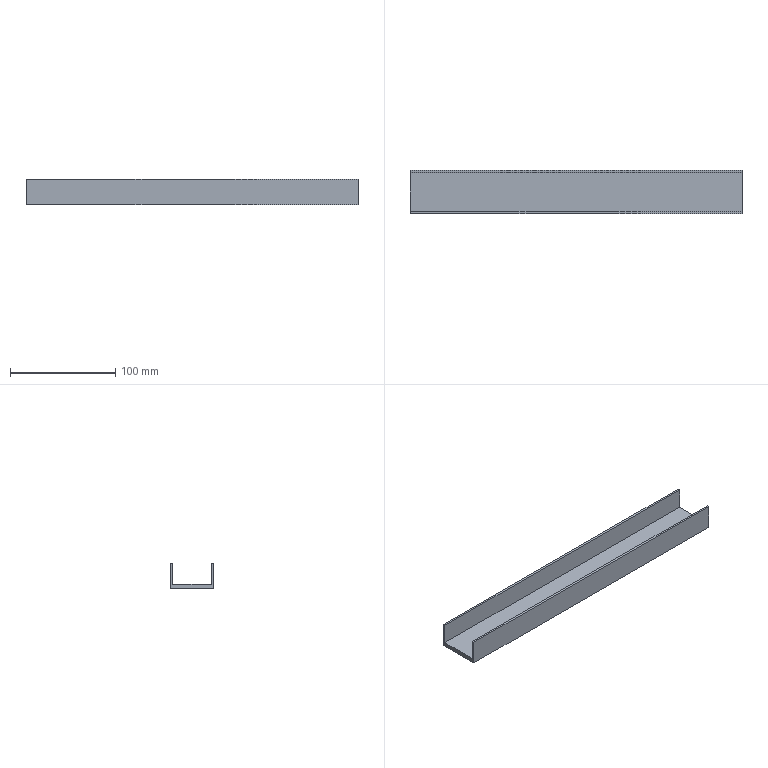Part | STEP file | Material chute | 1 solid | 10 faces | box 315 x 41 x 24 mm | volume 76860 mm3 | plane 10
STEP:
#1=CARTESIAN_POINT('',(190.,4.5,0.));
#2=VERTEX_POINT('',#1);
#3=CARTESIAN_POINT('',(190.,45.5,0.));
#4=VERTEX_POINT('',#3);
#5=CARTESIAN_POINT('',(190.,45.5,0.));
#6=DIRECTION('',(0.,1.,0.));
#7=VECTOR('',#6,1000.);
#8=LINE('',#5,#7);
#9=EDGE_CURVE('',#2,#4,#8,.T.);
#10=ORIENTED_EDGE('',*,*,#9,.T.);
#11=CARTESIAN_POINT('',(190.,45.5,24.));
#12=VERTEX_POINT('',#11);
#13=CARTESIAN_POINT('',(190.,45.5,4.));
#14=DIRECTION('',(0.,0.,-1.));
#15=VECTOR('',#14,1000.);
#16=LINE('',#13,#15);
#17=EDGE_CURVE('',#12,#4,#16,.T.);
#18=ORIENTED_EDGE('',*,*,#17,.F.);
#19=CARTESIAN_POINT('',(190.,43.5,24.));
#20=VERTEX_POINT('',#19);
#21=CARTESIAN_POINT('',(190.,45.5,24.));
#22=DIRECTION('',(0.,-1.,0.));
#23=VECTOR('',#22,1000.);
#24=LINE('',#21,#23);
#25=EDGE_CURVE('',#12,#20,#24,.T.);
#26=ORIENTED_EDGE('',*,*,#25,.T.);
#27=CARTESIAN_POINT('',(190.,43.5,4.));
#28=VERTEX_POINT('',#27);
#29=CARTESIAN_POINT('',(190.,43.5,24.));
#30=DIRECTION('',(0.,0.,-1.));
#31=VECTOR('',#30,1000.);
#32=LINE('',#29,#31);
#33=EDGE_CURVE('',#20,#28,#32,.T.);
#34=ORIENTED_EDGE('',*,*,#33,.T.);
#35=CARTESIAN_POINT('',(190.,6.5,4.));
#36=VERTEX_POINT('',#35);
#37=CARTESIAN_POINT('',(190.,45.5,4.));
#38=DIRECTION('',(0.,1.,0.));
#39=VECTOR('',#38,1000.);
#40=LINE('',#37,#39);
#41=EDGE_CURVE('',#36,#28,#40,.T.);
#42=ORIENTED_EDGE('',*,*,#41,.F.);
#43=CARTESIAN_POINT('',(190.,6.5,24.));
#44=VERTEX_POINT('',#43);
#45=CARTESIAN_POINT('',(190.,6.5,24.));
#46=DIRECTION('',(0.,0.,1.));
#47=VECTOR('',#46,1000.);
#48=LINE('',#45,#47);
#49=EDGE_CURVE('',#36,#44,#48,.T.);
#50=ORIENTED_EDGE('',*,*,#49,.T.);
#51=CARTESIAN_POINT('',(190.,4.5,24.));
#52=VERTEX_POINT('',#51);
#53=CARTESIAN_POINT('',(190.,4.5,24.));
#54=DIRECTION('',(0.,-1.,0.));
#55=VECTOR('',#54,1000.);
#56=LINE('',#53,#55);
#57=EDGE_CURVE('',#44,#52,#56,.T.);
#58=ORIENTED_EDGE('',*,*,#57,.T.);
#59=CARTESIAN_POINT('',(190.,4.5,4.));
#60=DIRECTION('',(0.,0.,-1.));
#61=VECTOR('',#60,1000.);
#62=LINE('',#59,#61);
#63=EDGE_CURVE('',#52,#2,#62,.T.);
#64=ORIENTED_EDGE('',*,*,#63,.T.);
#65=EDGE_LOOP('',(#10,#18,#26,#34,#42,#50,#58,#64));
#66=FACE_OUTER_BOUND('',#65,.T.);
#67=CARTESIAN_POINT('',(190.,45.5,4.));
#68=DIRECTION('',(-1.,0.,0.));
#69=DIRECTION('',(0.,0.,1.));
#70=AXIS2_PLACEMENT_3D('',#67,#68,#69);
#71=PLANE('',#70);
#72=ADVANCED_FACE('',(#66),#71,.F.);
#73=CARTESIAN_POINT('',(-125.,45.5,0.));
#74=VERTEX_POINT('',#73);
#75=CARTESIAN_POINT('',(190.,45.5,0.));
#76=DIRECTION('',(-1.,0.,0.));
#77=VECTOR('',#76,1000.);
#78=LINE('',#75,#77);
#79=EDGE_CURVE('',#4,#74,#78,.T.);
#80=ORIENTED_EDGE('',*,*,#79,.T.);
#81=CARTESIAN_POINT('',(-125.,45.5,24.));
#82=VERTEX_POINT('',#81);
#83=CARTESIAN_POINT('',(-125.,45.5,4.));
#84=DIRECTION('',(0.,0.,-1.));
#85=VECTOR('',#84,1000.);
#86=LINE('',#83,#85);
#87=EDGE_CURVE('',#82,#74,#86,.T.);
#88=ORIENTED_EDGE('',*,*,#87,.F.);
#89=CARTESIAN_POINT('',(210.1,45.5,24.));
#90=DIRECTION('',(-1.,0.,0.));
#91=VECTOR('',#90,1000.);
#92=LINE('',#89,#91);
#93=EDGE_CURVE('',#12,#82,#92,.T.);
#94=ORIENTED_EDGE('',*,*,#93,.F.);
#95=ORIENTED_EDGE('',*,*,#17,.T.);
#96=EDGE_LOOP('',(#80,#88,#94,#95));
#97=FACE_OUTER_BOUND('',#96,.T.);
#98=CARTESIAN_POINT('',(190.,45.5,4.));
#99=DIRECTION('',(0.,-1.,0.));
#100=DIRECTION('',(1.,0.,0.));
#101=AXIS2_PLACEMENT_3D('',#98,#99,#100);
#102=PLANE('',#101);
#103=ADVANCED_FACE('',(#97),#102,.F.);
#104=CARTESIAN_POINT('',(-125.,4.5,0.));
#105=VERTEX_POINT('',#104);
#106=CARTESIAN_POINT('',(-125.,45.5,0.));
#107=DIRECTION('',(0.,-1.,0.));
#108=VECTOR('',#107,1000.);
#109=LINE('',#106,#108);
#110=EDGE_CURVE('',#74,#105,#109,.T.);
#111=ORIENTED_EDGE('',*,*,#110,.T.);
#112=CARTESIAN_POINT('',(-125.,4.5,24.));
#113=VERTEX_POINT('',#112);
#114=CARTESIAN_POINT('',(-125.,4.5,4.));
#115=DIRECTION('',(0.,0.,-1.));
#116=VECTOR('',#115,1000.);
#117=LINE('',#114,#116);
#118=EDGE_CURVE('',#113,#105,#117,.T.);
#119=ORIENTED_EDGE('',*,*,#118,.F.);
#120=CARTESIAN_POINT('',(-125.,6.5,24.));
#121=VERTEX_POINT('',#120);
#122=CARTESIAN_POINT('',(-125.,4.5,24.));
#123=DIRECTION('',(0.,1.,0.));
#124=VECTOR('',#123,1000.);
#125=LINE('',#122,#124);
#126=EDGE_CURVE('',#113,#121,#125,.T.);
#127=ORIENTED_EDGE('',*,*,#126,.T.);
#128=CARTESIAN_POINT('',(-125.,6.5,4.));
#129=VERTEX_POINT('',#128);
#130=CARTESIAN_POINT('',(-125.,6.5,24.));
#131=DIRECTION('',(0.,0.,-1.));
#132=VECTOR('',#131,1000.);
#133=LINE('',#130,#132);
#134=EDGE_CURVE('',#121,#129,#133,.T.);
#135=ORIENTED_EDGE('',*,*,#134,.T.);
#136=CARTESIAN_POINT('',(-125.,43.5,4.));
#137=VERTEX_POINT('',#136);
#138=CARTESIAN_POINT('',(-125.,45.5,4.));
#139=DIRECTION('',(0.,-1.,0.));
#140=VECTOR('',#139,1000.);
#141=LINE('',#138,#140);
#142=EDGE_CURVE('',#137,#129,#141,.T.);
#143=ORIENTED_EDGE('',*,*,#142,.F.);
#144=CARTESIAN_POINT('',(-125.,43.5,24.));
#145=VERTEX_POINT('',#144);
#146=CARTESIAN_POINT('',(-125.,43.5,24.));
#147=DIRECTION('',(0.,0.,1.));
#148=VECTOR('',#147,1000.);
#149=LINE('',#146,#148);
#150=EDGE_CURVE('',#137,#145,#149,.T.);
#151=ORIENTED_EDGE('',*,*,#150,.T.);
#152=CARTESIAN_POINT('',(-125.,45.5,24.));
#153=DIRECTION('',(0.,1.,0.));
#154=VECTOR('',#153,1000.);
#155=LINE('',#152,#154);
#156=EDGE_CURVE('',#145,#82,#155,.T.);
#157=ORIENTED_EDGE('',*,*,#156,.T.);
#158=ORIENTED_EDGE('',*,*,#87,.T.);
#159=EDGE_LOOP('',(#111,#119,#127,#135,#143,#151,#157,#158));
#160=FACE_OUTER_BOUND('',#159,.T.);
#161=CARTESIAN_POINT('',(-125.,45.5,4.));
#162=DIRECTION('',(1.,0.,0.));
#163=DIRECTION('',(0.,0.,-1.));
#164=AXIS2_PLACEMENT_3D('',#161,#162,#163);
#165=PLANE('',#164);
#166=ADVANCED_FACE('',(#160),#165,.F.);
#167=CARTESIAN_POINT('',(190.,4.5,0.));
#168=DIRECTION('',(1.,0.,0.));
#169=VECTOR('',#168,1000.);
#170=LINE('',#167,#169);
#171=EDGE_CURVE('',#105,#2,#170,.T.);
#172=ORIENTED_EDGE('',*,*,#171,.T.);
#173=ORIENTED_EDGE('',*,*,#63,.F.);
#174=CARTESIAN_POINT('',(210.1,4.5,24.));
#175=DIRECTION('',(-1.,0.,0.));
#176=VECTOR('',#175,1000.);
#177=LINE('',#174,#176);
#178=EDGE_CURVE('',#52,#113,#177,.T.);
#179=ORIENTED_EDGE('',*,*,#178,.T.);
#180=ORIENTED_EDGE('',*,*,#118,.T.);
#181=EDGE_LOOP('',(#172,#173,#179,#180));
#182=FACE_OUTER_BOUND('',#181,.T.);
#183=CARTESIAN_POINT('',(190.,4.5,4.));
#184=DIRECTION('',(0.,1.,0.));
#185=DIRECTION('',(-1.,0.,0.));
#186=AXIS2_PLACEMENT_3D('',#183,#184,#185);
#187=PLANE('',#186);
#188=ADVANCED_FACE('',(#182),#187,.F.);
#189=ORIENTED_EDGE('',*,*,#142,.T.);
#190=CARTESIAN_POINT('',(210.1,6.5,4.));
#191=DIRECTION('',(-1.,0.,0.));
#192=VECTOR('',#191,1000.);
#193=LINE('',#190,#192);
#194=EDGE_CURVE('',#36,#129,#193,.T.);
#195=ORIENTED_EDGE('',*,*,#194,.F.);
#196=ORIENTED_EDGE('',*,*,#41,.T.);
#197=CARTESIAN_POINT('',(210.1,43.5,4.));
#198=DIRECTION('',(-1.,0.,0.));
#199=VECTOR('',#198,1000.);
#200=LINE('',#197,#199);
#201=EDGE_CURVE('',#28,#137,#200,.T.);
#202=ORIENTED_EDGE('',*,*,#201,.T.);
#203=EDGE_LOOP('',(#189,#195,#196,#202));
#204=FACE_OUTER_BOUND('',#203,.T.);
#205=CARTESIAN_POINT('',(0.,0.,4.));
#206=DIRECTION('',(0.,0.,-1.));
#207=DIRECTION('',(-1.,0.,0.));
#208=AXIS2_PLACEMENT_3D('',#205,#206,#207);
#209=PLANE('',#208);
#210=ADVANCED_FACE('',(#204),#209,.F.);
#211=ORIENTED_EDGE('',*,*,#9,.F.);
#212=ORIENTED_EDGE('',*,*,#171,.F.);
#213=ORIENTED_EDGE('',*,*,#110,.F.);
#214=ORIENTED_EDGE('',*,*,#79,.F.);
#215=EDGE_LOOP('',(#211,#212,#213,#214));
#216=FACE_OUTER_BOUND('',#215,.T.);
#217=CARTESIAN_POINT('',(0.,0.,0.));
#218=DIRECTION('',(0.,0.,-1.));
#219=DIRECTION('',(-1.,0.,0.));
#220=AXIS2_PLACEMENT_3D('',#217,#218,#219);
#221=PLANE('',#220);
#222=ADVANCED_FACE('',(#216),#221,.T.);
#223=ORIENTED_EDGE('',*,*,#25,.F.);
#224=ORIENTED_EDGE('',*,*,#93,.T.);
#225=ORIENTED_EDGE('',*,*,#156,.F.);
#226=CARTESIAN_POINT('',(210.1,43.5,24.));
#227=DIRECTION('',(-1.,0.,0.));
#228=VECTOR('',#227,1000.);
#229=LINE('',#226,#228);
#230=EDGE_CURVE('',#20,#145,#229,.T.);
#231=ORIENTED_EDGE('',*,*,#230,.F.);
#232=EDGE_LOOP('',(#223,#224,#225,#231));
#233=FACE_OUTER_BOUND('',#232,.T.);
#234=CARTESIAN_POINT('',(210.1,45.5,24.));
#235=DIRECTION('',(0.,0.,1.));
#236=DIRECTION('',(1.,0.,0.));
#237=AXIS2_PLACEMENT_3D('',#234,#235,#236);
#238=PLANE('',#237);
#239=ADVANCED_FACE('',(#233),#238,.T.);
#240=ORIENTED_EDGE('',*,*,#33,.F.);
#241=ORIENTED_EDGE('',*,*,#230,.T.);
#242=ORIENTED_EDGE('',*,*,#150,.F.);
#243=ORIENTED_EDGE('',*,*,#201,.F.);
#244=EDGE_LOOP('',(#240,#241,#242,#243));
#245=FACE_OUTER_BOUND('',#244,.T.);
#246=CARTESIAN_POINT('',(210.1,43.5,24.));
#247=DIRECTION('',(0.,-1.,0.));
#248=DIRECTION('',(1.,0.,0.));
#249=AXIS2_PLACEMENT_3D('',#246,#247,#248);
#250=PLANE('',#249);
#251=ADVANCED_FACE('',(#245),#250,.T.);
#252=ORIENTED_EDGE('',*,*,#49,.F.);
#253=ORIENTED_EDGE('',*,*,#194,.T.);
#254=ORIENTED_EDGE('',*,*,#134,.F.);
#255=CARTESIAN_POINT('',(210.1,6.5,24.));
#256=DIRECTION('',(-1.,0.,0.));
#257=VECTOR('',#256,1000.);
#258=LINE('',#255,#257);
#259=EDGE_CURVE('',#44,#121,#258,.T.);
#260=ORIENTED_EDGE('',*,*,#259,.F.);
#261=EDGE_LOOP('',(#252,#253,#254,#260));
#262=FACE_OUTER_BOUND('',#261,.T.);
#263=CARTESIAN_POINT('',(210.1,6.5,24.));
#264=DIRECTION('',(0.,1.,0.));
#265=DIRECTION('',(-1.,0.,0.));
#266=AXIS2_PLACEMENT_3D('',#263,#264,#265);
#267=PLANE('',#266);
#268=ADVANCED_FACE('',(#262),#267,.T.);
#269=ORIENTED_EDGE('',*,*,#57,.F.);
#270=ORIENTED_EDGE('',*,*,#259,.T.);
#271=ORIENTED_EDGE('',*,*,#126,.F.);
#272=ORIENTED_EDGE('',*,*,#178,.F.);
#273=EDGE_LOOP('',(#269,#270,#271,#272));
#274=FACE_OUTER_BOUND('',#273,.T.);
#275=CARTESIAN_POINT('',(210.1,4.5,24.));
#276=DIRECTION('',(0.,0.,1.));
#277=DIRECTION('',(1.,0.,0.));
#278=AXIS2_PLACEMENT_3D('',#275,#276,#277);
#279=PLANE('',#278);
#280=ADVANCED_FACE('',(#274),#279,.T.);
#281=CLOSED_SHELL('',(#72,#103,#166,#188,#210,#222,#239,#251,#268,#280));
#282=MANIFOLD_SOLID_BREP('',#281);
#283=CARTESIAN_POINT('',(0.,0.,0.));
#284=DIRECTION('',(0.,0.,1.));
#285=DIRECTION('',(1.,0.,0.));
#286=AXIS2_PLACEMENT_3D('',#283,#284,#285);
#287=(LENGTH_UNIT()NAMED_UNIT(*)SI_UNIT(.MILLI.,.METRE.));
#288=UNCERTAINTY_MEASURE_WITH_UNIT(LENGTH_MEASURE(0.00001),#287,'','');
#289=(NAMED_UNIT(*)PLANE_ANGLE_UNIT()SI_UNIT($,.RADIAN.));
#290=(NAMED_UNIT(*)SI_UNIT($,.STERADIAN.)SOLID_ANGLE_UNIT());
#291=(GEOMETRIC_REPRESENTATION_CONTEXT(3)GLOBAL_UNCERTAINTY_ASSIGNED_CONTEXT((#288))GLOBAL_UNIT_ASSIGNED_CONTEXT((#287,#289,#290))REPRESENTATION_CONTEXT('',''));
#292=ADVANCED_BREP_SHAPE_REPRESENTATION('',(#282,#286),#291);